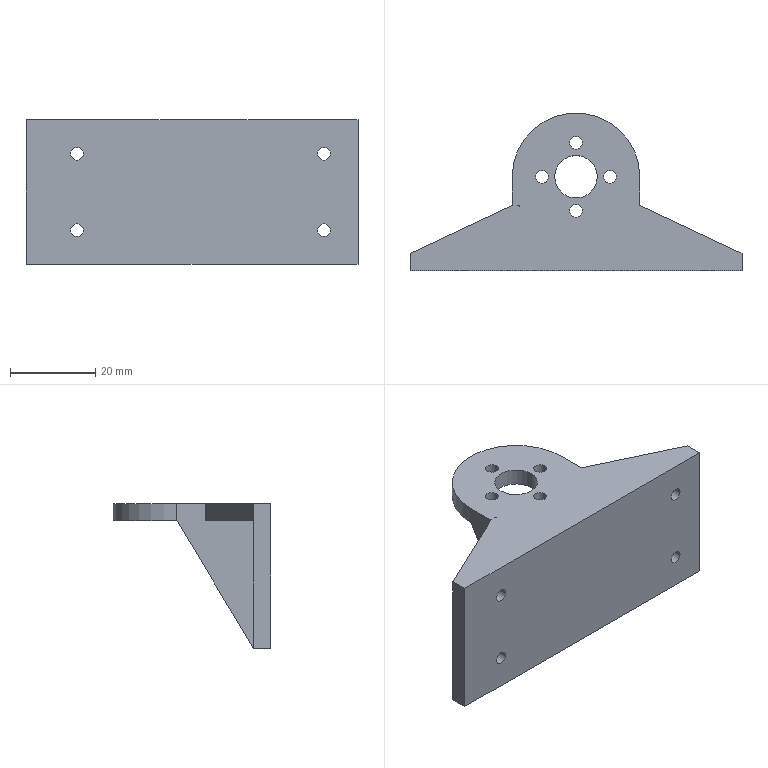Part | STEP file | Lead screw push block | 1 solid | 42 faces | box 78 x 37 x 34 mm | volume 16349 mm3 | plane 22 | cylinder 20 | commonest cylinder face diameters 3 x16 10 x2 30 x2